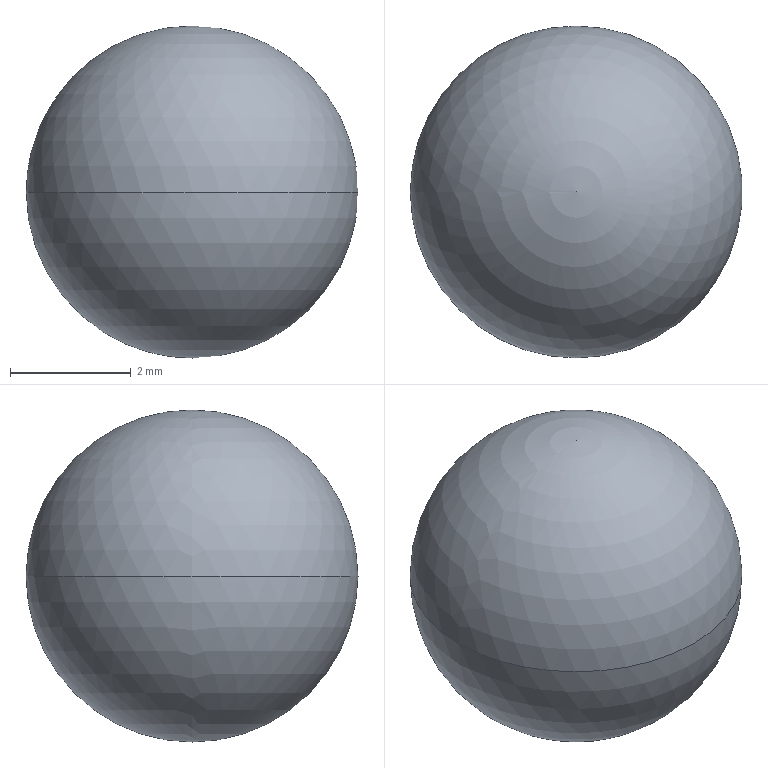Part | SolidWorks | features Revolution 1 | 1 solid | 2 faces | box 5.5 x 5.5 x 5.5 mm | volume 87.114 mm3 | sphere 2
STEP:
#1=CARTESIAN_POINT('',(0.,5.5,0.));
#2=VERTEX_POINT('',#1);
#3=CARTESIAN_POINT('',(0.,0.,0.));
#4=VERTEX_POINT('',#3);
#5=CARTESIAN_POINT('',(0.,2.75,0.));
#6=DIRECTION('',(0.,0.,1.));
#7=DIRECTION('',(1.,0.,0.));
#8=AXIS2_PLACEMENT_3D('',#5,#6,#7);
#9=CIRCLE('',#8,2.75);
#10=EDGE_CURVE('',#2,#4,#9,.T.);
#11=ORIENTED_EDGE('',*,*,#10,.F.);
#12=CARTESIAN_POINT('',(0.,2.75,0.));
#13=DIRECTION('',(0.,0.,-1.));
#14=DIRECTION('',(-1.,0.,0.));
#15=AXIS2_PLACEMENT_3D('',#12,#13,#14);
#16=CIRCLE('',#15,2.75);
#17=EDGE_CURVE('',#2,#4,#16,.T.);
#18=ORIENTED_EDGE('',*,*,#17,.T.);
#19=EDGE_LOOP('',(#11,#18));
#20=FACE_OUTER_BOUND('',#19,.T.);
#21=CARTESIAN_POINT('',(0.,2.75,0.));
#22=DIRECTION('',(0.,0.,-1.));
#23=DIRECTION('',(-1.,0.,0.));
#24=AXIS2_PLACEMENT_3D('',#21,#22,#23);
#25=SPHERICAL_SURFACE('',#24,2.75);
#26=ADVANCED_FACE('',(#20),#25,.T.);
#27=ORIENTED_EDGE('',*,*,#17,.F.);
#28=ORIENTED_EDGE('',*,*,#10,.T.);
#29=EDGE_LOOP('',(#27,#28));
#30=FACE_OUTER_BOUND('',#29,.T.);
#31=CARTESIAN_POINT('',(0.,2.75,0.));
#32=DIRECTION('',(0.,0.,-1.));
#33=DIRECTION('',(-1.,0.,0.));
#34=AXIS2_PLACEMENT_3D('',#31,#32,#33);
#35=SPHERICAL_SURFACE('',#34,2.75);
#36=ADVANCED_FACE('',(#30),#35,.T.);
#37=CLOSED_SHELL('',(#26,#36));
#38=MANIFOLD_SOLID_BREP('',#37);
#39=CARTESIAN_POINT('',(0.,0.,0.));
#40=DIRECTION('',(0.,0.,1.));
#41=DIRECTION('',(1.,0.,0.));
#42=AXIS2_PLACEMENT_3D('',#39,#40,#41);
#43=(LENGTH_UNIT()NAMED_UNIT(*)SI_UNIT(.MILLI.,.METRE.));
#44=UNCERTAINTY_MEASURE_WITH_UNIT(LENGTH_MEASURE(0.00001),#43,'','');
#45=(NAMED_UNIT(*)PLANE_ANGLE_UNIT()SI_UNIT($,.RADIAN.));
#46=(NAMED_UNIT(*)SI_UNIT($,.STERADIAN.)SOLID_ANGLE_UNIT());
#47=(GEOMETRIC_REPRESENTATION_CONTEXT(3)GLOBAL_UNCERTAINTY_ASSIGNED_CONTEXT((#44))GLOBAL_UNIT_ASSIGNED_CONTEXT((#43,#45,#46))REPRESENTATION_CONTEXT('',''));
#48=ADVANCED_BREP_SHAPE_REPRESENTATION('',(#38,#42),#47);